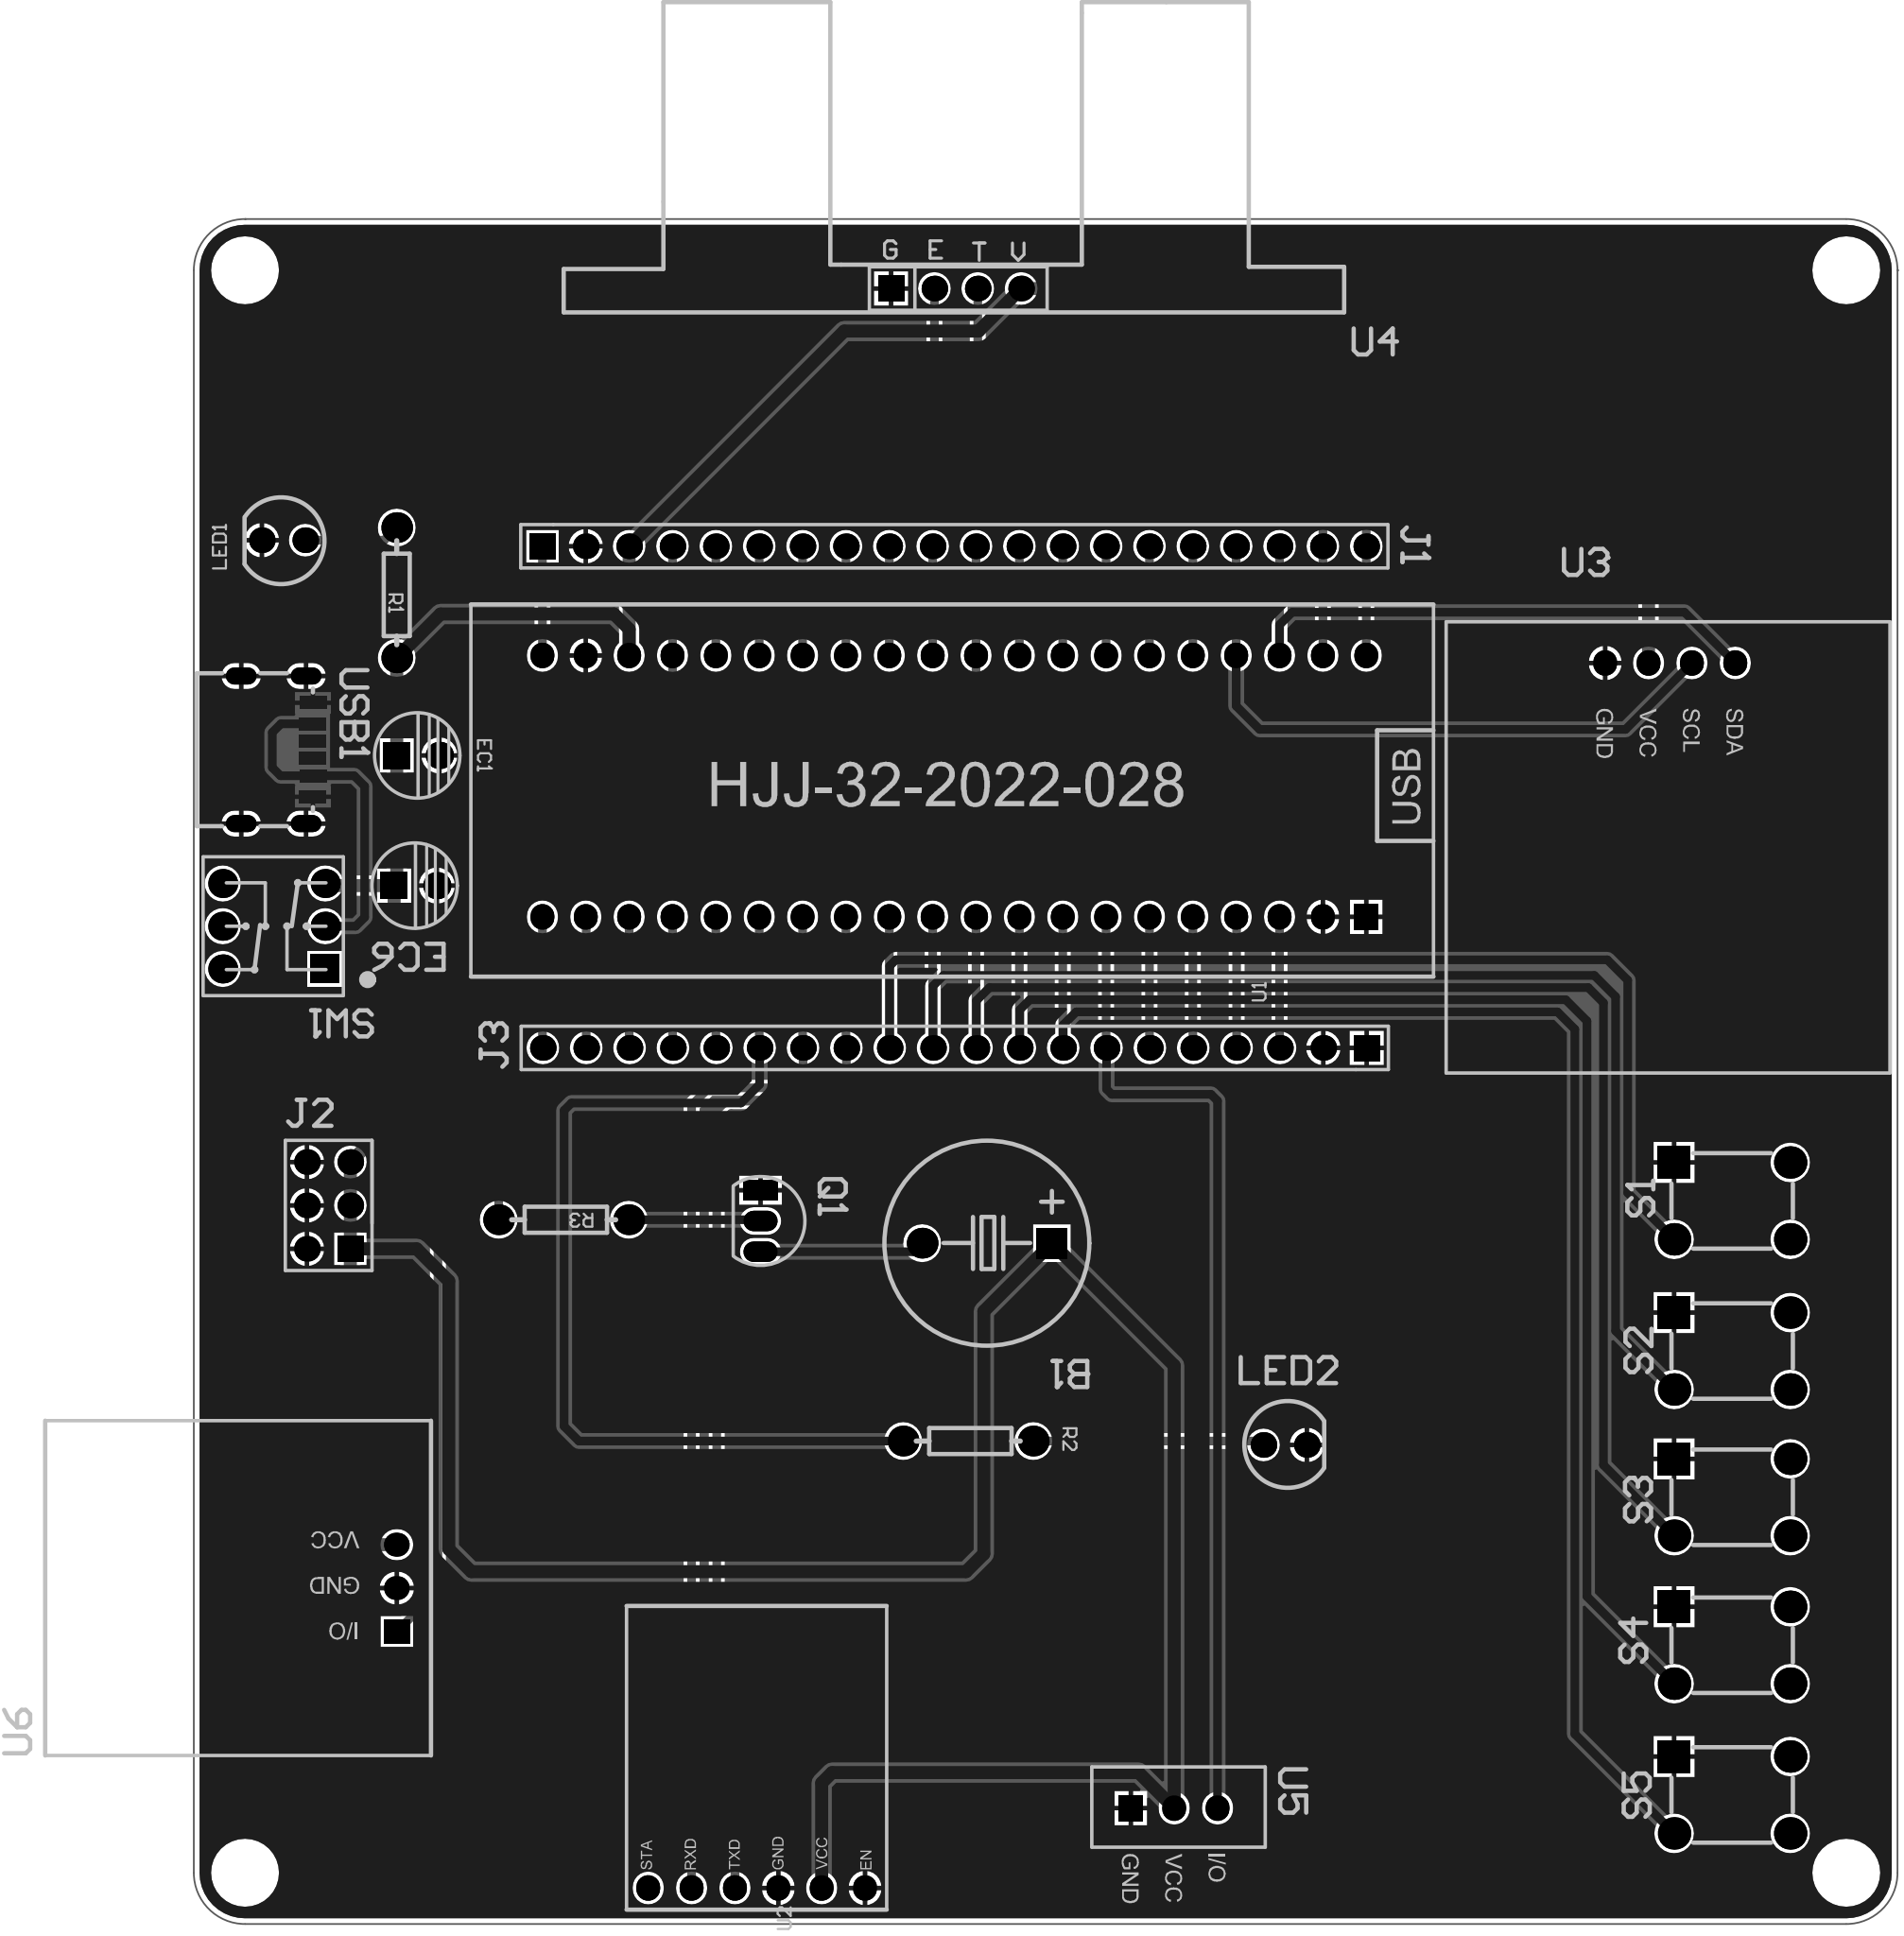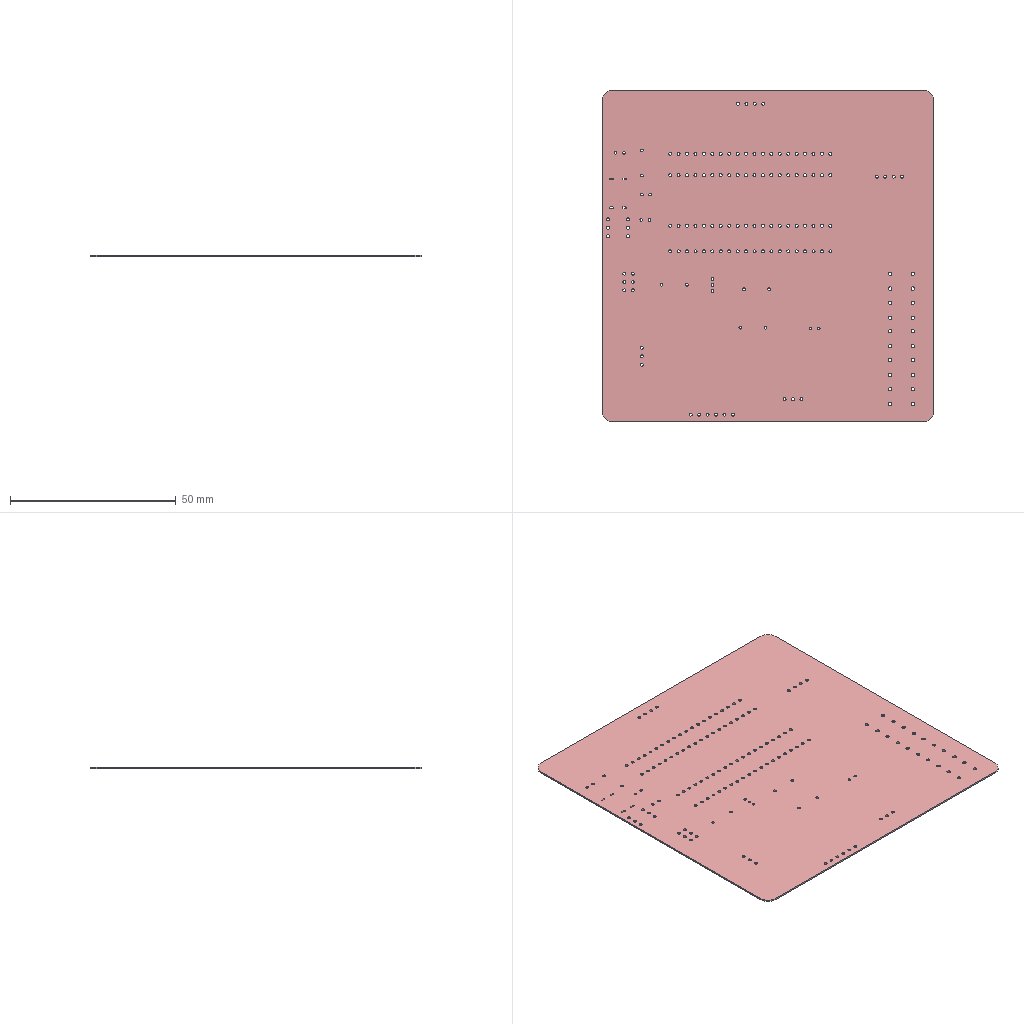Circuit board layout | Altium Designer | box 99.8 x 99.8 x 0.5 mm
Layer stack:
# Altium Designer layer stack of  (unit mm; dielectric type: 0 none, 1 core, 2 prepreg, 3 surface material)
index,name,kind,layer,copper_thickness_mm,dielectric_type,dielectric_thickness_mm,dielectric_material,dielectric_constant
0,Top Paste Mask Layer,other,,,,,,
1,Top Silkscreen Layer,other,,,,,,
2,Top Solder Mask Layer,dielectric,,,3,0.0356,FR-4,4.8
3,Top Layer,copper,Top Layer,0.0356,,,,
4,Substrate1,dielectric,,,3,0.32,FR-4,4.8
5,Bottom Layer,copper,Bottom Layer,0.0356,,,,
6,Bottom Solder Mask Layer,dielectric,,,3,0.0356,FR-4,4.8
7,Bottom Silkscreen Layer,other,,,,,,
8,Bottom Paste Mask Layer,other,,,,,,
# drill layer pairs: low layer,high layer
drill_pair,Top Layer,Bottom Layer
Part placement:
Designator,Comment,Layer,Footprint,Center-X(mm),Center-Y(mm),Rotation
USB1,TYPEC-250D-BCP6,TopLayer,TYP-C-6,94.412,153.772,270
SW1,KFT DIP-8X8,TopLayer,KFT_DIP-8X8,94.231,143.445,180
J3,,TopLayer,Pin_HDR1X20/2.54mm-S,134.112,136.322,180
J2,Pin HDR2X3,TopLayer,Pin_HDR2X3/2.54mm-S,97.434,127.102,90
J1,,TopLayer,Pin_HDR1X20/2.54mm-S,134.087,165.684,0
EC6,10uF,TopLayer,DIP-EC2.5X5X11,102.52,145.821,0
EC1,220uF,TopLayer,DIP-EC2.5X5X11,102.672,153.441,0
LED1,LED,TopLayer,LED5-BLUE,94.793,166.04,180
R1,1k,TopLayer,AXIAL0.3,101.422,162.966,270
R2,k?,TopLayer,AXIAL0.3,134.899,113.309,0
R3,1K,TopLayer,AXIAL0.3,111.201,126.263,0
U1,STM32F103,TopLayer,STM32FF103,134.087,151.643,90
U2,ESP8266,TopLayer,ECB02,122.504,87.147,90
B1,BEEP,TopLayer,BEEP_7.6X12X7.5,136.002,124.892,180
LED2,LED,TopLayer,LED5-BLUE,153.467,113.081,0
Q1,NPN,TopLayer,TO-92A,122.733,126.191,270
S1,BUTTOM,TopLayer,DIP-6X6X5,179.651,127.366,0
S2,BUTTOM,TopLayer,DIP-6X6X5,179.651,118.578,0
S3,BUTTOM,TopLayer,DIP-6X6X5,179.651,110.018,0
S4,BUTTOM,TopLayer,DIP-6X6X5,179.651,101.357,0
S5,BUTTOM,TopLayer,DIP-6X6X5,179.651,92.594,0
U3,OLED,TopLayer,OLED,176.022,158.852,270
U4,HC-SR04,TopLayer,超声波MODE,134.188,180.772,0
U5,SG90,TopLayer,SG90,146.964,91.821,270
U6,Infrared pair,TopLayer,红外对管,101.429,104.703,180
Pad and via stacks:
# Altium Designer via and pad stacks of  (unit mm). Each distinct definition once, with the count of objects using it.
# via: kind,start_layer,end_layer,hole_mm,diameter_mm,mode(0 simple;1 top-mid-bottom;2 full stack),diameter_per_layer,count,example_net
# pad: kind,layer,hole_mm,hole_type(0 round;1 square;2 slot),plating,top_size,top_shape(1 round;2 rect;3 octagon;9 rounded rect),mid_size,bottom_size,mode,footprint,size_per_layer,count,example
pad,Multi-Layer,0.5,2,plated,1x1.8,1,1x1.8,1x1.8,0,TYP-C-6,,4,USB1.3
pad,Multi-Layer,0.9,0,plated,1.7x1.7,1,1.7x1.7,1.7x1.7,0,KFT DIP-8X8,,5,SW1.6
pad,Multi-Layer,0.9,0,plated,1.7x1.7,2,1.7x1.7,1.7x1.7,0,KFT DIP-8X8,,1,SW1.1
pad,Multi-Layer,0.9,0,plated,1.5x1.5,2,1.5x1.5,1.5x1.5,0,Pin HDR1X20/2.54mm-S,,2,J3.1
pad,Multi-Layer,0.9,0,plated,1.5x1.5,1,1.5x1.5,1.5x1.5,0,Pin HDR1X20/2.54mm-S,,38,J3.2
pad,Multi-Layer,0.9,0,plated,1.5x1.5,1,1.5x1.5,1.5x1.5,0,Pin HDR2X3/2.54mm-S,,5,J2.6
pad,Multi-Layer,0.9,0,plated,1.5x1.5,2,1.5x1.5,1.5x1.5,0,Pin HDR2X3/2.54mm-S,,1,J2.1
pad,Multi-Layer,0.8,0,plated,1.6x1.6,2,1.6x1.6,1.6x1.6,0,DIP-EC2.5X5X11,,2,EC6.1
pad,Multi-Layer,0.8,0,plated,1.6x1.6,1,1.6x1.6,1.6x1.6,0,DIP-EC2.5X5X11,,2,EC6.2
pad,Multi-Layer,0.762,0,plated,1.5x1.5,1,1.5x1.5,1.5x1.5,0,LED5-BLUE,,4,LED1.K
pad,Multi-Layer,0.8,0,plated,1.8x1.8,1,1.8x1.8,1.8x1.8,0,AXIAL0.3,,6,R1.2
pad,Multi-Layer,0.9,0,plated,1.4x1.5,1,1.4x1.5,1.4x1.5,0,STM32FF103,,39,U1.27
pad,Multi-Layer,0.9,0,plated,1.4x1.5,2,1.4x1.5,1.4x1.5,0,STM32FF103,,1,U1.1
pad,Multi-Layer,0.9,0,plated,1.4x1.5,1,1.4x1.5,1.4x1.5,0,ECB02,,6,U2.4
pad,Multi-Layer,0.9,0,plated,1.8x1.8,2,1.8x1.8,1.8x1.8,0,BEEP 7.6X12X7.5,,1,B1.1
pad,Multi-Layer,0.9,0,plated,1.8x1.8,1,1.8x1.8,1.8x1.8,0,BEEP 7.6X12X7.5,,1,B1.2
pad,Multi-Layer,0.8,0,plated,2x1.2,1,2x1.2,2x1.2,0,TO-92A,,2,Q1.C
pad,Multi-Layer,0.8,0,plated,2x1.2,2,2x1.2,2x1.2,0,TO-92A,,1,Q1.E
pad,Multi-Layer,1,0,plated,1.9x1.9,2,1.9x1.9,1.9x1.9,0,DIP-6X6X5,,5,S1.1
pad,Multi-Layer,1,0,plated,1.9x1.9,1,1.9x1.9,1.9x1.9,0,DIP-6X6X5,,15,S1.2
pad,Multi-Layer,0.9,0,plated,1.4x1.5,1,1.4x1.5,1.4x1.5,0,OLED,,4,U3.4
pad,Multi-Layer,0.85,0,plated,1.5x1.5,2,1.5x1.5,1.5x1.5,0,\u00B3\u00AC\u00C9\u00F9\u00B2\u00A8MODE,,1,U4.1
pad,Multi-Layer,0.85,0,plated,1.5x1.5,1,1.5x1.5,1.5x1.5,0,\u00B3\u00AC\u00C9\u00F9\u00B2\u00A8MODE,,3,U4.2
pad,Multi-Layer,0.9,0,plated,1.4x1.5,2,1.4x1.5,1.4x1.5,0,SG90,,1,U5.1
pad,Multi-Layer,0.9,0,plated,1.4x1.5,1,1.4x1.5,1.4x1.5,0,SG90,,2,U5.2
pad,Multi-Layer,0.9,0,plated,1.4x1.5,1,1.4x1.5,1.4x1.5,0,\u00BA\u00EC\u00CD\u00E2\u00B6\u00D4\u00B9\u00DC,,2,U6.3
pad,Multi-Layer,0.9,0,plated,1.4x1.5,2,1.4x1.5,1.4x1.5,0,\u00BA\u00EC\u00CD\u00E2\u00B6\u00D4\u00B9\u00DC,,1,U6.1
pad,Top Layer,0,0,plated,0.75x1.6,2,0.75x1.6,0.75x1.6,0,TYP-C-6,,6,USB1.A12
Copper pours:
name,layer,net,type(0 solid;1 hatched;2 none)
Top Layer-GND,Top Layer,GND,0
Bottom Layer-GND,Bottom Layer,GND,0
Design rules, without the lines most boards share:
# Altium Designer design rules of  (exported by Altium Designer, unit mm)
# columns: name | kind | enabled | priority | scope1 | scope2 | descriptor | typed fields (field=value)
ComponentClearance_1 | 24 | enabled | 1 | All | All | Component Clearance Constraint ( Horizontal Gap = 10mil, Vertical Gap = 10mil ) (All),(All)  | gap=0.254
Clearance | 0 | enabled | 1 | All | All | Clearance Constraint (Gap=8mil) (All),(All) | gap=0.2032
Clearance_1 | 63 | enabled | 1 | All | All | Board Clearance Constraint (Gap=0mil) (All) |
ComponentClearance | 52 | enabled | 1 | All | All | Hole To Hole Clearance (Gap=10mil) (All),(All) | gap=0.254
Width | 2 | enabled | 1 | All | All | Width Constraint (Min=20mil) (Max=30mil) (Preferred=20mil) (All) |
DiffPairsRouting | 51 | enabled | 1 | All | All | Differential Pairs Uncoupled Length using the Gap Constraints (Min=10mil) (Max=10mil) (Prefered=10mil)  and Width Constraints (Min=99999mil) (Max=0mil) (Prefered=0mil) (All) |
RoutingVias | 11 | enabled | 1 | All | All | Routing Via (MinHoleWidth=11.811mil) (MaxHoleWidth=11.811mil) (PreferredHoleWidth=11.811mil) (MinWidth=23.622mil) (MaxWidth=23.622mil) (PreferedWidth=23.622mil) (All) | via_min_hole=0.3 via_max_hole=0.3 via_preferred_diameter=0.6 via_preferred_hole=0.3
PlaneConnect | 6 | enabled | 1 | All | All | Power Plane Connect Rule(Relief Connect )(Expansion=20mil) (Conductor Width=10mil) (Air Gap=10mil) (Entries=4) (All) | relief_conductor_width=0.254 relief_entries=4 relief_expansion=0.508
PolygonConnect | 20 | enabled | 1 | All | All | Polygon Connect Rule(Relief Connect )(Conductor Width=10mil) (Relief Angle=90 Angle) (Entries=4) (Air Gap Width=10mil) (All),(All) | connect_style(0=relief,1=direct,2=none)=0 relief_conductor_width=0.254 relief_entries=4
PasteMaskExpansion | 14 | enabled | 1 | All | All | Paste Mask Expansion (Expansion =0mil) (All) | expansion=0
SolderMaskExpansion | 13 | enabled | 1 | All | All | Solder Mask Expansion (Expansion =4mil) (All) | expansion=0.1016